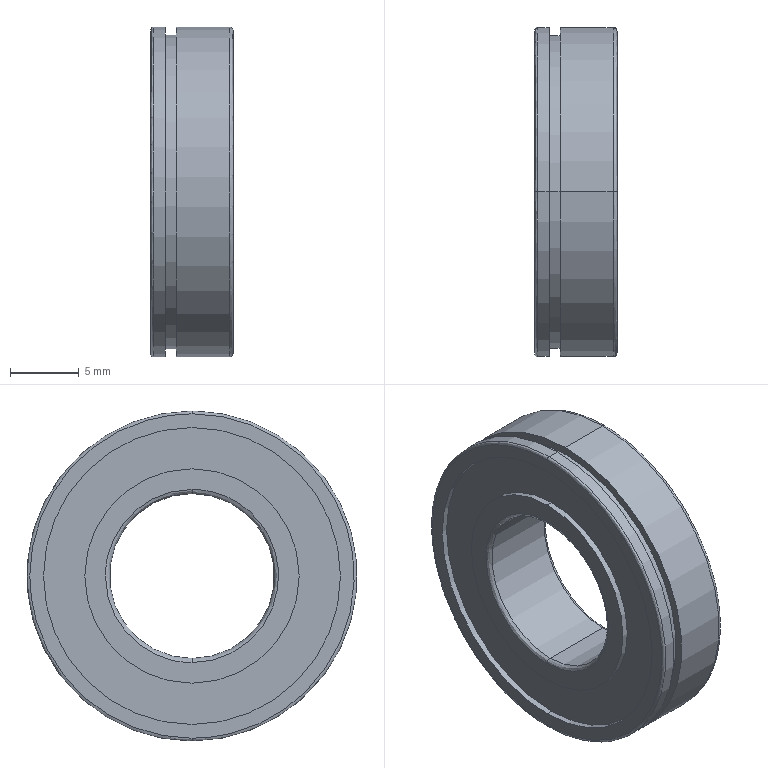Part | STEP file | 0243_Z_B6901ZZNR_1 | 1 solid | 32 faces | box 6 x 24 x 24 mm | volume 1839 mm3 | cylinder 16 | spline 8 | plane 8 | commonest cylinder face diameters 15.6 x4 21.6 x4 24 x4 12 x2 22.8 x2